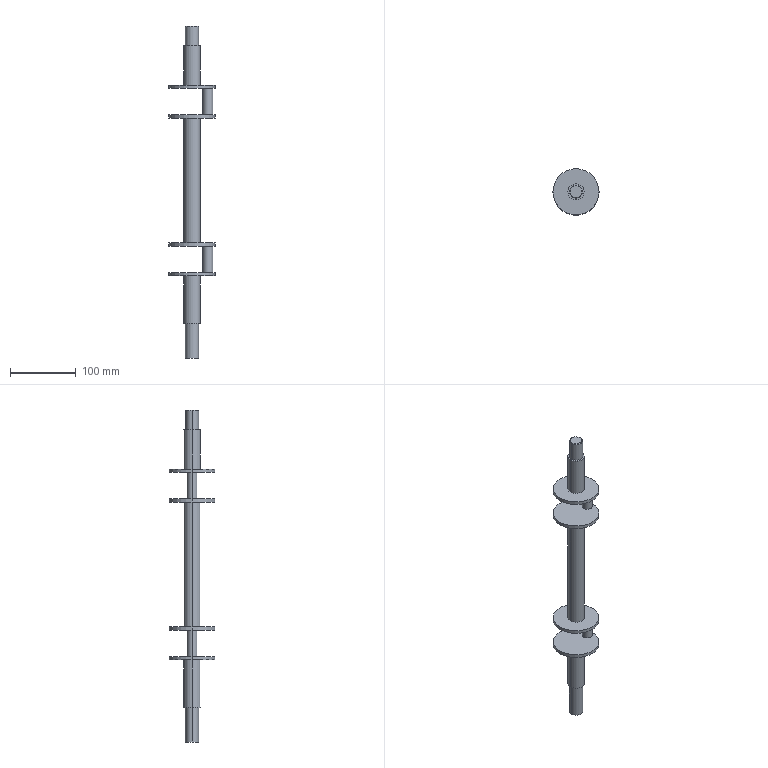Part | SolidWorks | features BaseBody 1 | 1 solid | 36 faces | box 70 x 70 x 505 mm | volume 275389 mm3 | cylinder 22 | plane 12 | cone 2 | commonest cylinder face diameters 70 x8 25 x6 15 x4 20 x4
STEP:
#1=CARTESIAN_POINT('',(10.,0.,30.));
#2=VERTEX_POINT('',#1);
#3=CARTESIAN_POINT('',(-10.,0.,30.));
#4=VERTEX_POINT('',#3);
#5=CARTESIAN_POINT('',(0.,0.,30.));
#6=DIRECTION('',(0.,0.,-1.));
#7=DIRECTION('',(1.,0.,0.));
#8=AXIS2_PLACEMENT_3D('',#5,#6,#7);
#9=CIRCLE('',#8,10.);
#10=EDGE_CURVE('',#2,#4,#9,.T.);
#11=ORIENTED_EDGE('',*,*,#10,.T.);
#12=CARTESIAN_POINT('',(-10.,0.,-22.));
#13=VERTEX_POINT('',#12);
#14=CARTESIAN_POINT('',(-10.,0.,0.));
#15=DIRECTION('',(0.,0.,-1.));
#16=VECTOR('',#15,1000.);
#17=LINE('',#14,#16);
#18=EDGE_CURVE('',#4,#13,#17,.T.);
#19=ORIENTED_EDGE('',*,*,#18,.T.);
#20=CARTESIAN_POINT('',(10.,0.,-22.));
#21=VERTEX_POINT('',#20);
#22=CARTESIAN_POINT('',(0.,0.,-22.));
#23=DIRECTION('',(0.,0.,-1.));
#24=DIRECTION('',(1.,0.,0.));
#25=AXIS2_PLACEMENT_3D('',#22,#23,#24);
#26=CIRCLE('',#25,10.);
#27=EDGE_CURVE('',#21,#13,#26,.T.);
#28=ORIENTED_EDGE('',*,*,#27,.F.);
#29=CARTESIAN_POINT('',(10.,0.,0.));
#30=DIRECTION('',(0.,0.,-1.));
#31=VECTOR('',#30,1000.);
#32=LINE('',#29,#31);
#33=EDGE_CURVE('',#2,#21,#32,.T.);
#34=ORIENTED_EDGE('',*,*,#33,.F.);
#35=EDGE_LOOP('',(#11,#19,#28,#34));
#36=FACE_OUTER_BOUND('',#35,.T.);
#37=CARTESIAN_POINT('',(0.,0.,0.));
#38=DIRECTION('',(0.,0.,-1.));
#39=DIRECTION('',(1.,0.,0.));
#40=AXIS2_PLACEMENT_3D('',#37,#38,#39);
#41=CYLINDRICAL_SURFACE('',#40,10.);
#42=ADVANCED_FACE('',(#36),#41,.T.);
#43=CARTESIAN_POINT('',(-9.,0.,483.));
#44=VERTEX_POINT('',#43);
#45=CARTESIAN_POINT('',(9.,0.,483.));
#46=VERTEX_POINT('',#45);
#47=CARTESIAN_POINT('',(0.,0.,483.));
#48=DIRECTION('',(0.,0.,-1.));
#49=DIRECTION('',(-1.,0.,0.));
#50=AXIS2_PLACEMENT_3D('',#47,#48,#49);
#51=CIRCLE('',#50,9.);
#52=EDGE_CURVE('',#44,#46,#51,.T.);
#53=ORIENTED_EDGE('',*,*,#52,.T.);
#54=CARTESIAN_POINT('',(10.,0.,482.));
#55=VERTEX_POINT('',#54);
#56=CARTESIAN_POINT('',(9.5,0.,482.5));
#57=DIRECTION('',(0.7071,0.,-0.7071));
#58=VECTOR('',#57,1000.);
#59=LINE('',#56,#58);
#60=EDGE_CURVE('',#46,#55,#59,.T.);
#61=ORIENTED_EDGE('',*,*,#60,.T.);
#62=CARTESIAN_POINT('',(-10.,0.,482.));
#63=VERTEX_POINT('',#62);
#64=CARTESIAN_POINT('',(0.,0.,482.));
#65=DIRECTION('',(0.,0.,1.));
#66=DIRECTION('',(-1.,0.,0.));
#67=AXIS2_PLACEMENT_3D('',#64,#65,#66);
#68=CIRCLE('',#67,10.);
#69=EDGE_CURVE('',#55,#63,#68,.T.);
#70=ORIENTED_EDGE('',*,*,#69,.T.);
#71=CARTESIAN_POINT('',(-9.5,0.,482.5));
#72=DIRECTION('',(-0.7071,0.,-0.7071));
#73=VECTOR('',#72,1000.);
#74=LINE('',#71,#73);
#75=EDGE_CURVE('',#44,#63,#74,.T.);
#76=ORIENTED_EDGE('',*,*,#75,.F.);
#77=EDGE_LOOP('',(#53,#61,#70,#76));
#78=FACE_OUTER_BOUND('',#77,.T.);
#79=CARTESIAN_POINT('',(0.,0.,482.5));
#80=DIRECTION('',(0.,0.,-1.));
#81=DIRECTION('',(-1.,0.,0.));
#82=AXIS2_PLACEMENT_3D('',#79,#80,#81);
#83=CONICAL_SURFACE('',#82,9.5,0.7854);
#84=ADVANCED_FACE('',(#78),#83,.T.);
#85=CARTESIAN_POINT('',(-10.,0.,453.));
#86=VERTEX_POINT('',#85);
#87=CARTESIAN_POINT('',(10.,0.,453.));
#88=VERTEX_POINT('',#87);
#89=CARTESIAN_POINT('',(0.,0.,453.));
#90=DIRECTION('',(0.,0.,1.));
#91=DIRECTION('',(-1.,0.,0.));
#92=AXIS2_PLACEMENT_3D('',#89,#90,#91);
#93=CIRCLE('',#92,10.);
#94=EDGE_CURVE('',#86,#88,#93,.T.);
#95=ORIENTED_EDGE('',*,*,#94,.T.);
#96=CARTESIAN_POINT('',(10.,0.,483.));
#97=DIRECTION('',(0.,0.,1.));
#98=VECTOR('',#97,1000.);
#99=LINE('',#96,#98);
#100=EDGE_CURVE('',#88,#55,#99,.T.);
#101=ORIENTED_EDGE('',*,*,#100,.T.);
#102=CARTESIAN_POINT('',(0.,0.,482.));
#103=DIRECTION('',(0.,0.,1.));
#104=DIRECTION('',(-1.,0.,0.));
#105=AXIS2_PLACEMENT_3D('',#102,#103,#104);
#106=CIRCLE('',#105,10.);
#107=EDGE_CURVE('',#63,#55,#106,.T.);
#108=ORIENTED_EDGE('',*,*,#107,.F.);
#109=CARTESIAN_POINT('',(-10.,0.,483.));
#110=DIRECTION('',(0.,0.,1.));
#111=VECTOR('',#110,1000.);
#112=LINE('',#109,#111);
#113=EDGE_CURVE('',#86,#63,#112,.T.);
#114=ORIENTED_EDGE('',*,*,#113,.F.);
#115=EDGE_LOOP('',(#95,#101,#108,#114));
#116=FACE_OUTER_BOUND('',#115,.T.);
#117=CARTESIAN_POINT('',(0.,0.,483.));
#118=DIRECTION('',(0.,0.,1.));
#119=DIRECTION('',(-1.,0.,0.));
#120=AXIS2_PLACEMENT_3D('',#117,#118,#119);
#121=CYLINDRICAL_SURFACE('',#120,10.);
#122=ADVANCED_FACE('',(#116),#121,.T.);
#123=CARTESIAN_POINT('',(-12.5,0.,453.));
#124=VERTEX_POINT('',#123);
#125=CARTESIAN_POINT('',(12.5,0.,453.));
#126=VERTEX_POINT('',#125);
#127=CARTESIAN_POINT('',(0.,0.,453.));
#128=DIRECTION('',(0.,0.,-1.));
#129=DIRECTION('',(-1.,0.,0.));
#130=AXIS2_PLACEMENT_3D('',#127,#128,#129);
#131=CIRCLE('',#130,12.5);
#132=EDGE_CURVE('',#124,#126,#131,.T.);
#133=ORIENTED_EDGE('',*,*,#132,.T.);
#134=CARTESIAN_POINT('',(12.5,0.,393.));
#135=VERTEX_POINT('',#134);
#136=CARTESIAN_POINT('',(12.5,0.,393.));
#137=DIRECTION('',(0.,0.,-1.));
#138=VECTOR('',#137,1000.);
#139=LINE('',#136,#138);
#140=EDGE_CURVE('',#126,#135,#139,.T.);
#141=ORIENTED_EDGE('',*,*,#140,.T.);
#142=CARTESIAN_POINT('',(-12.5,0.,393.));
#143=VERTEX_POINT('',#142);
#144=CARTESIAN_POINT('',(0.,0.,393.));
#145=DIRECTION('',(0.,0.,-1.));
#146=DIRECTION('',(-1.,0.,0.));
#147=AXIS2_PLACEMENT_3D('',#144,#145,#146);
#148=CIRCLE('',#147,12.5);
#149=EDGE_CURVE('',#143,#135,#148,.T.);
#150=ORIENTED_EDGE('',*,*,#149,.F.);
#151=CARTESIAN_POINT('',(-12.5,0.,393.));
#152=DIRECTION('',(0.,0.,-1.));
#153=VECTOR('',#152,1000.);
#154=LINE('',#151,#153);
#155=EDGE_CURVE('',#124,#143,#154,.T.);
#156=ORIENTED_EDGE('',*,*,#155,.F.);
#157=EDGE_LOOP('',(#133,#141,#150,#156));
#158=FACE_OUTER_BOUND('',#157,.T.);
#159=CARTESIAN_POINT('',(0.,0.,393.));
#160=DIRECTION('',(0.,0.,-1.));
#161=DIRECTION('',(-1.,0.,0.));
#162=AXIS2_PLACEMENT_3D('',#159,#160,#161);
#163=CYLINDRICAL_SURFACE('',#162,12.5);
#164=ADVANCED_FACE('',(#158),#163,.T.);
#165=CARTESIAN_POINT('',(35.,0.,393.));
#166=VERTEX_POINT('',#165);
#167=CARTESIAN_POINT('',(-35.,0.,393.));
#168=VERTEX_POINT('',#167);
#169=CARTESIAN_POINT('',(0.,0.,393.));
#170=DIRECTION('',(0.,0.,1.));
#171=DIRECTION('',(-1.,0.,0.));
#172=AXIS2_PLACEMENT_3D('',#169,#170,#171);
#173=CIRCLE('',#172,35.);
#174=EDGE_CURVE('',#166,#168,#173,.T.);
#175=ORIENTED_EDGE('',*,*,#174,.F.);
#176=CARTESIAN_POINT('',(35.,0.,388.));
#177=VERTEX_POINT('',#176);
#178=CARTESIAN_POINT('',(35.,0.,388.));
#179=DIRECTION('',(0.,0.,-1.));
#180=VECTOR('',#179,1000.);
#181=LINE('',#178,#180);
#182=EDGE_CURVE('',#166,#177,#181,.T.);
#183=ORIENTED_EDGE('',*,*,#182,.T.);
#184=CARTESIAN_POINT('',(-35.,0.,388.));
#185=VERTEX_POINT('',#184);
#186=CARTESIAN_POINT('',(0.,0.,388.));
#187=DIRECTION('',(0.,0.,-1.));
#188=DIRECTION('',(-1.,0.,0.));
#189=AXIS2_PLACEMENT_3D('',#186,#187,#188);
#190=CIRCLE('',#189,35.);
#191=EDGE_CURVE('',#185,#177,#190,.T.);
#192=ORIENTED_EDGE('',*,*,#191,.F.);
#193=CARTESIAN_POINT('',(-35.,0.,388.));
#194=DIRECTION('',(0.,0.,-1.));
#195=VECTOR('',#194,1000.);
#196=LINE('',#193,#195);
#197=EDGE_CURVE('',#168,#185,#196,.T.);
#198=ORIENTED_EDGE('',*,*,#197,.F.);
#199=EDGE_LOOP('',(#175,#183,#192,#198));
#200=FACE_OUTER_BOUND('',#199,.T.);
#201=CARTESIAN_POINT('',(0.,0.,388.));
#202=DIRECTION('',(0.,0.,-1.));
#203=DIRECTION('',(-1.,0.,0.));
#204=AXIS2_PLACEMENT_3D('',#201,#202,#203);
#205=CYLINDRICAL_SURFACE('',#204,35.);
#206=ADVANCED_FACE('',(#200),#205,.T.);
#207=CARTESIAN_POINT('',(31.5,0.,388.));
#208=VERTEX_POINT('',#207);
#209=CARTESIAN_POINT('',(16.5,0.,388.));
#210=VERTEX_POINT('',#209);
#211=CARTESIAN_POINT('',(24.,0.,388.));
#212=DIRECTION('',(0.,0.,1.));
#213=DIRECTION('',(-1.,0.,0.));
#214=AXIS2_PLACEMENT_3D('',#211,#212,#213);
#215=CIRCLE('',#214,7.5);
#216=EDGE_CURVE('',#208,#210,#215,.T.);
#217=ORIENTED_EDGE('',*,*,#216,.F.);
#218=CARTESIAN_POINT('',(31.5,0.,348.));
#219=VERTEX_POINT('',#218);
#220=CARTESIAN_POINT('',(31.5,0.,348.));
#221=DIRECTION('',(0.,0.,-1.));
#222=VECTOR('',#221,1000.);
#223=LINE('',#220,#222);
#224=EDGE_CURVE('',#208,#219,#223,.T.);
#225=ORIENTED_EDGE('',*,*,#224,.T.);
#226=CARTESIAN_POINT('',(16.5,0.,348.));
#227=VERTEX_POINT('',#226);
#228=CARTESIAN_POINT('',(24.,0.,348.));
#229=DIRECTION('',(0.,0.,-1.));
#230=DIRECTION('',(-1.,0.,0.));
#231=AXIS2_PLACEMENT_3D('',#228,#229,#230);
#232=CIRCLE('',#231,7.5);
#233=EDGE_CURVE('',#227,#219,#232,.T.);
#234=ORIENTED_EDGE('',*,*,#233,.F.);
#235=CARTESIAN_POINT('',(16.5,0.,348.));
#236=DIRECTION('',(0.,0.,-1.));
#237=VECTOR('',#236,1000.);
#238=LINE('',#235,#237);
#239=EDGE_CURVE('',#210,#227,#238,.T.);
#240=ORIENTED_EDGE('',*,*,#239,.F.);
#241=EDGE_LOOP('',(#217,#225,#234,#240));
#242=FACE_OUTER_BOUND('',#241,.T.);
#243=CARTESIAN_POINT('',(24.,0.,348.));
#244=DIRECTION('',(0.,0.,-1.));
#245=DIRECTION('',(-1.,0.,0.));
#246=AXIS2_PLACEMENT_3D('',#243,#244,#245);
#247=CYLINDRICAL_SURFACE('',#246,7.5);
#248=ADVANCED_FACE('',(#242),#247,.T.);
#249=CARTESIAN_POINT('',(35.,0.,348.));
#250=VERTEX_POINT('',#249);
#251=CARTESIAN_POINT('',(-35.,0.,348.));
#252=VERTEX_POINT('',#251);
#253=CARTESIAN_POINT('',(0.,0.,348.));
#254=DIRECTION('',(0.,0.,1.));
#255=DIRECTION('',(-1.,0.,0.));
#256=AXIS2_PLACEMENT_3D('',#253,#254,#255);
#257=CIRCLE('',#256,35.);
#258=EDGE_CURVE('',#250,#252,#257,.T.);
#259=ORIENTED_EDGE('',*,*,#258,.F.);
#260=CARTESIAN_POINT('',(35.,0.,343.));
#261=VERTEX_POINT('',#260);
#262=CARTESIAN_POINT('',(35.,0.,343.));
#263=DIRECTION('',(0.,0.,-1.));
#264=VECTOR('',#263,1000.);
#265=LINE('',#262,#264);
#266=EDGE_CURVE('',#250,#261,#265,.T.);
#267=ORIENTED_EDGE('',*,*,#266,.T.);
#268=CARTESIAN_POINT('',(-35.,0.,343.));
#269=VERTEX_POINT('',#268);
#270=CARTESIAN_POINT('',(0.,0.,343.));
#271=DIRECTION('',(0.,0.,-1.));
#272=DIRECTION('',(-1.,0.,0.));
#273=AXIS2_PLACEMENT_3D('',#270,#271,#272);
#274=CIRCLE('',#273,35.);
#275=EDGE_CURVE('',#269,#261,#274,.T.);
#276=ORIENTED_EDGE('',*,*,#275,.F.);
#277=CARTESIAN_POINT('',(-35.,0.,343.));
#278=DIRECTION('',(0.,0.,-1.));
#279=VECTOR('',#278,1000.);
#280=LINE('',#277,#279);
#281=EDGE_CURVE('',#252,#269,#280,.T.);
#282=ORIENTED_EDGE('',*,*,#281,.F.);
#283=EDGE_LOOP('',(#259,#267,#276,#282));
#284=FACE_OUTER_BOUND('',#283,.T.);
#285=CARTESIAN_POINT('',(0.,0.,343.));
#286=DIRECTION('',(0.,0.,-1.));
#287=DIRECTION('',(-1.,0.,0.));
#288=AXIS2_PLACEMENT_3D('',#285,#286,#287);
#289=CYLINDRICAL_SURFACE('',#288,35.);
#290=ADVANCED_FACE('',(#284),#289,.T.);
#291=CARTESIAN_POINT('',(12.5,0.,343.));
#292=VERTEX_POINT('',#291);
#293=CARTESIAN_POINT('',(-12.5,0.,343.));
#294=VERTEX_POINT('',#293);
#295=CARTESIAN_POINT('',(0.,0.,343.));
#296=DIRECTION('',(0.,0.,1.));
#297=DIRECTION('',(-1.,0.,0.));
#298=AXIS2_PLACEMENT_3D('',#295,#296,#297);
#299=CIRCLE('',#298,12.5);
#300=EDGE_CURVE('',#292,#294,#299,.T.);
#301=ORIENTED_EDGE('',*,*,#300,.F.);
#302=CARTESIAN_POINT('',(12.5,0.,153.));
#303=VERTEX_POINT('',#302);
#304=CARTESIAN_POINT('',(12.5,0.,153.));
#305=DIRECTION('',(0.,0.,-1.));
#306=VECTOR('',#305,1000.);
#307=LINE('',#304,#306);
#308=EDGE_CURVE('',#292,#303,#307,.T.);
#309=ORIENTED_EDGE('',*,*,#308,.T.);
#310=CARTESIAN_POINT('',(-12.5,0.,153.));
#311=VERTEX_POINT('',#310);
#312=CARTESIAN_POINT('',(0.,0.,153.));
#313=DIRECTION('',(0.,0.,-1.));
#314=DIRECTION('',(-1.,0.,0.));
#315=AXIS2_PLACEMENT_3D('',#312,#313,#314);
#316=CIRCLE('',#315,12.5);
#317=EDGE_CURVE('',#311,#303,#316,.T.);
#318=ORIENTED_EDGE('',*,*,#317,.F.);
#319=CARTESIAN_POINT('',(-12.5,0.,153.));
#320=DIRECTION('',(0.,0.,-1.));
#321=VECTOR('',#320,1000.);
#322=LINE('',#319,#321);
#323=EDGE_CURVE('',#294,#311,#322,.T.);
#324=ORIENTED_EDGE('',*,*,#323,.F.);
#325=EDGE_LOOP('',(#301,#309,#318,#324));
#326=FACE_OUTER_BOUND('',#325,.T.);
#327=CARTESIAN_POINT('',(0.,0.,153.));
#328=DIRECTION('',(0.,0.,-1.));
#329=DIRECTION('',(-1.,0.,0.));
#330=AXIS2_PLACEMENT_3D('',#327,#328,#329);
#331=CYLINDRICAL_SURFACE('',#330,12.5);
#332=ADVANCED_FACE('',(#326),#331,.T.);
#333=CARTESIAN_POINT('',(35.,0.,153.));
#334=VERTEX_POINT('',#333);
#335=CARTESIAN_POINT('',(-35.,0.,153.));
#336=VERTEX_POINT('',#335);
#337=CARTESIAN_POINT('',(0.,0.,153.));
#338=DIRECTION('',(0.,0.,1.));
#339=DIRECTION('',(-1.,0.,0.));
#340=AXIS2_PLACEMENT_3D('',#337,#338,#339);
#341=CIRCLE('',#340,35.);
#342=EDGE_CURVE('',#334,#336,#341,.T.);
#343=ORIENTED_EDGE('',*,*,#342,.F.);
#344=CARTESIAN_POINT('',(35.,0.,148.));
#345=VERTEX_POINT('',#344);
#346=CARTESIAN_POINT('',(35.,0.,148.));
#347=DIRECTION('',(0.,0.,-1.));
#348=VECTOR('',#347,1000.);
#349=LINE('',#346,#348);
#350=EDGE_CURVE('',#334,#345,#349,.T.);
#351=ORIENTED_EDGE('',*,*,#350,.T.);
#352=CARTESIAN_POINT('',(-35.,0.,148.));
#353=VERTEX_POINT('',#352);
#354=CARTESIAN_POINT('',(0.,0.,148.));
#355=DIRECTION('',(0.,0.,-1.));
#356=DIRECTION('',(-1.,0.,0.));
#357=AXIS2_PLACEMENT_3D('',#354,#355,#356);
#358=CIRCLE('',#357,35.);
#359=EDGE_CURVE('',#353,#345,#358,.T.);
#360=ORIENTED_EDGE('',*,*,#359,.F.);
#361=CARTESIAN_POINT('',(-35.,0.,148.));
#362=DIRECTION('',(0.,0.,-1.));
#363=VECTOR('',#362,1000.);
#364=LINE('',#361,#363);
#365=EDGE_CURVE('',#336,#353,#364,.T.);
#366=ORIENTED_EDGE('',*,*,#365,.F.);
#367=EDGE_LOOP('',(#343,#351,#360,#366));
#368=FACE_OUTER_BOUND('',#367,.T.);
#369=CARTESIAN_POINT('',(0.,0.,148.));
#370=DIRECTION('',(0.,0.,-1.));
#371=DIRECTION('',(-1.,0.,0.));
#372=AXIS2_PLACEMENT_3D('',#369,#370,#371);
#373=CYLINDRICAL_SURFACE('',#372,35.);
#374=ADVANCED_FACE('',(#368),#373,.T.);
#375=CARTESIAN_POINT('',(31.5,0.,148.));
#376=VERTEX_POINT('',#375);
#377=CARTESIAN_POINT('',(16.5,0.,148.));
#378=VERTEX_POINT('',#377);
#379=CARTESIAN_POINT('',(24.,0.,148.));
#380=DIRECTION('',(0.,0.,1.));
#381=DIRECTION('',(-1.,0.,0.));
#382=AXIS2_PLACEMENT_3D('',#379,#380,#381);
#383=CIRCLE('',#382,7.5);
#384=EDGE_CURVE('',#376,#378,#383,.T.);
#385=ORIENTED_EDGE('',*,*,#384,.F.);
#386=CARTESIAN_POINT('',(31.5,0.,108.));
#387=VERTEX_POINT('',#386);
#388=CARTESIAN_POINT('',(31.5,0.,108.));
#389=DIRECTION('',(0.,0.,-1.));
#390=VECTOR('',#389,1000.);
#391=LINE('',#388,#390);
#392=EDGE_CURVE('',#376,#387,#391,.T.);
#393=ORIENTED_EDGE('',*,*,#392,.T.);
#394=CARTESIAN_POINT('',(16.5,0.,108.));
#395=VERTEX_POINT('',#394);
#396=CARTESIAN_POINT('',(24.,0.,108.));
#397=DIRECTION('',(0.,0.,-1.));
#398=DIRECTION('',(-1.,0.,0.));
#399=AXIS2_PLACEMENT_3D('',#396,#397,#398);
#400=CIRCLE('',#399,7.5);
#401=EDGE_CURVE('',#395,#387,#400,.T.);
#402=ORIENTED_EDGE('',*,*,#401,.F.);
#403=CARTESIAN_POINT('',(16.5,0.,108.));
#404=DIRECTION('',(0.,0.,-1.));
#405=VECTOR('',#404,1000.);
#406=LINE('',#403,#405);
#407=EDGE_CURVE('',#378,#395,#406,.T.);
#408=ORIENTED_EDGE('',*,*,#407,.F.);
#409=EDGE_LOOP('',(#385,#393,#402,#408));
#410=FACE_OUTER_BOUND('',#409,.T.);
#411=CARTESIAN_POINT('',(24.,0.,108.));
#412=DIRECTION('',(0.,0.,-1.));
#413=DIRECTION('',(-1.,0.,0.));
#414=AXIS2_PLACEMENT_3D('',#411,#412,#413);
#415=CYLINDRICAL_SURFACE('',#414,7.5);
#416=ADVANCED_FACE('',(#410),#415,.T.);
#417=CARTESIAN_POINT('',(35.,0.,108.));
#418=VERTEX_POINT('',#417);
#419=CARTESIAN_POINT('',(-35.,0.,108.));
#420=VERTEX_POINT('',#419);
#421=CARTESIAN_POINT('',(0.,0.,108.));
#422=DIRECTION('',(0.,0.,1.));
#423=DIRECTION('',(-1.,0.,0.));
#424=AXIS2_PLACEMENT_3D('',#421,#422,#423);
#425=CIRCLE('',#424,35.);
#426=EDGE_CURVE('',#418,#420,#425,.T.);
#427=ORIENTED_EDGE('',*,*,#426,.F.);
#428=CARTESIAN_POINT('',(35.,0.,103.));
#429=VERTEX_POINT('',#428);
#430=CARTESIAN_POINT('',(35.,0.,103.));
#431=DIRECTION('',(0.,0.,-1.));
#432=VECTOR('',#431,1000.);
#433=LINE('',#430,#432);
#434=EDGE_CURVE('',#418,#429,#433,.T.);
#435=ORIENTED_EDGE('',*,*,#434,.T.);
#436=CARTESIAN_POINT('',(-35.,0.,103.));
#437=VERTEX_POINT('',#436);
#438=CARTESIAN_POINT('',(0.,0.,103.));
#439=DIRECTION('',(0.,0.,-1.));
#440=DIRECTION('',(-1.,0.,0.));
#441=AXIS2_PLACEMENT_3D('',#438,#439,#440);
#442=CIRCLE('',#441,35.);
#443=EDGE_CURVE('',#437,#429,#442,.T.);
#444=ORIENTED_EDGE('',*,*,#443,.F.);
#445=CARTESIAN_POINT('',(-35.,0.,103.));
#446=DIRECTION('',(0.,0.,-1.));
#447=VECTOR('',#446,1000.);
#448=LINE('',#445,#447);
#449=EDGE_CURVE('',#420,#437,#448,.T.);
#450=ORIENTED_EDGE('',*,*,#449,.F.);
#451=EDGE_LOOP('',(#427,#435,#444,#450));
#452=FACE_OUTER_BOUND('',#451,.T.);
#453=CARTESIAN_POINT('',(0.,0.,103.));
#454=DIRECTION('',(0.,0.,-1.));
#455=DIRECTION('',(-1.,0.,0.));
#456=AXIS2_PLACEMENT_3D('',#453,#454,#455);
#457=CYLINDRICAL_SURFACE('',#456,35.);
#458=ADVANCED_FACE('',(#452),#457,.T.);
#459=CARTESIAN_POINT('',(12.5,0.,103.));
#460=VERTEX_POINT('',#459);
#461=CARTESIAN_POINT('',(-12.5,0.,103.));
#462=VERTEX_POINT('',#461);
#463=CARTESIAN_POINT('',(0.,0.,103.));
#464=DIRECTION('',(0.,0.,1.));
#465=DIRECTION('',(-1.,0.,0.));
#466=AXIS2_PLACEMENT_3D('',#463,#464,#465);
#467=CIRCLE('',#466,12.5);
#468=EDGE_CURVE('',#460,#462,#467,.T.);
#469=ORIENTED_EDGE('',*,*,#468,.F.);
#470=CARTESIAN_POINT('',(12.5,0.,30.));
#471=VERTEX_POINT('',#470);
#472=CARTESIAN_POINT('',(12.5,0.,0.));
#473=DIRECTION('',(0.,0.,-1.));
#474=VECTOR('',#473,1000.);
#475=LINE('',#472,#474);
#476=EDGE_CURVE('',#460,#471,#475,.T.);
#477=ORIENTED_EDGE('',*,*,#476,.T.);
#478=CARTESIAN_POINT('',(-12.5,0.,30.));
#479=VERTEX_POINT('',#478);
#480=CARTESIAN_POINT('',(0.,0.,30.));
#481=DIRECTION('',(0.,0.,1.));
#482=DIRECTION('',(-1.,0.,0.));
#483=AXIS2_PLACEMENT_3D('',#480,#481,#482);
#484=CIRCLE('',#483,12.5);
#485=EDGE_CURVE('',#471,#479,#484,.T.);
#486=ORIENTED_EDGE('',*,*,#485,.T.);
#487=CARTESIAN_POINT('',(-12.5,0.,0.));
#488=DIRECTION('',(0.,0.,-1.));
#489=VECTOR('',#488,1000.);
#490=LINE('',#487,#489);
#491=EDGE_CURVE('',#462,#479,#490,.T.);
#492=ORIENTED_EDGE('',*,*,#491,.F.);
#493=EDGE_LOOP('',(#469,#477,#486,#492));
#494=FACE_OUTER_BOUND('',#493,.T.);
#495=CARTESIAN_POINT('',(0.,0.,0.));
#496=DIRECTION('',(0.,0.,-1.));
#497=DIRECTION('',(-1.,0.,0.));
#498=AXIS2_PLACEMENT_3D('',#495,#496,#497);
#499=CYLINDRICAL_SURFACE('',#498,12.5);
#500=ADVANCED_FACE('',(#494),#499,.T.);
#501=ORIENTED_EDGE('',*,*,#27,.T.);
#502=CARTESIAN_POINT('',(0.,0.,-22.));
#503=DIRECTION('',(0.,0.,-1.));
#504=DIRECTION('',(1.,0.,0.));
#505=AXIS2_PLACEMENT_3D('',#502,#503,#504);
#506=CIRCLE('',#505,10.);
#507=EDGE_CURVE('',#13,#21,#506,.T.);
#508=ORIENTED_EDGE('',*,*,#507,.T.);
#509=EDGE_LOOP('',(#501,#508));
#510=FACE_OUTER_BOUND('',#509,.T.);
#511=CARTESIAN_POINT('',(0.,0.,-22.));
#512=DIRECTION('',(0.,0.,1.));
#513=DIRECTION('',(1.,0.,0.));
#514=AXIS2_PLACEMENT_3D('',#511,#512,#513);
#515=PLANE('',#514);
#516=ADVANCED_FACE('',(#510),#515,.F.);
#517=ORIENTED_EDGE('',*,*,#10,.F.);
#518=CARTESIAN_POINT('',(0.,0.,30.));
#519=DIRECTION('',(0.,0.,-1.));
#520=DIRECTION('',(1.,0.,0.));
#521=AXIS2_PLACEMENT_3D('',#518,#519,#520);
#522=CIRCLE('',#521,10.);
#523=EDGE_CURVE('',#4,#2,#522,.T.);
#524=ORIENTED_EDGE('',*,*,#523,.F.);
#525=EDGE_LOOP('',(#517,#524));
#526=FACE_BOUND('',#525,.T.);
#527=CARTESIAN_POINT('',(0.,0.,30.));
#528=DIRECTION('',(0.,0.,1.));
#529=DIRECTION('',(-1.,0.,0.));
#530=AXIS2_PLACEMENT_3D('',#527,#528,#529);
#531=CIRCLE('',#530,12.5);
#532=EDGE_CURVE('',#479,#471,#531,.T.);
#533=ORIENTED_EDGE('',*,*,#532,.F.);
#534=ORIENTED_EDGE('',*,*,#485,.F.);
#535=EDGE_LOOP('',(#533,#534));
#536=FACE_OUTER_BOUND('',#535,.T.);
#537=CARTESIAN_POINT('',(0.,0.,30.));
#538=DIRECTION('',(0.,0.,1.));
#539=DIRECTION('',(1.,0.,0.));
#540=AXIS2_PLACEMENT_3D('',#537,#538,#539);
#541=PLANE('',#540);
#542=ADVANCED_FACE('',(#526,#536),#541,.F.);
#543=ORIENTED_EDGE('',*,*,#52,.F.);
#544=CARTESIAN_POINT('',(0.,0.,483.));
#545=DIRECTION('',(0.,0.,-1.));
#546=DIRECTION('',(-1.,0.,0.));
#547=AXIS2_PLACEMENT_3D('',#544,#545,#546);
#548=CIRCLE('',#547,9.);
#549=EDGE_CURVE('',#46,#44,#548,.T.);
#550=ORIENTED_EDGE('',*,*,#549,.F.);
#551=EDGE_LOOP('',(#543,#550));
#552=FACE_OUTER_BOUND('',#551,.T.);
#553=CARTESIAN_POINT('',(0.,0.,483.));
#554=DIRECTION('',(0.,0.,1.));
#555=DIRECTION('',(1.,0.,0.));
#556=AXIS2_PLACEMENT_3D('',#553,#554,#555);
#557=PLANE('',#556);
#558=ADVANCED_FACE('',(#552),#557,.T.);
#559=ORIENTED_EDGE('',*,*,#94,.F.);
#560=CARTESIAN_POINT('',(0.,0.,453.));
#561=DIRECTION('',(0.,0.,1.));
#562=DIRECTION('',(-1.,0.,0.));
#563=AXIS2_PLACEMENT_3D('',#560,#561,#562);
#564=CIRCLE('',#563,10.);
#565=EDGE_CURVE('',#88,#86,#564,.T.);
#566=ORIENTED_EDGE('',*,*,#565,.F.);
#567=EDGE_LOOP('',(#559,#566));
#568=FACE_BOUND('',#567,.T.);
#569=ORIENTED_EDGE('',*,*,#132,.F.);
#570=CARTESIAN_POINT('',(0.,0.,453.));
#571=DIRECTION('',(0.,0.,-1.));
#572=DIRECTION('',(-1.,0.,0.));
#573=AXIS2_PLACEMENT_3D('',#570,#571,#572);
#574=CIRCLE('',#573,12.5);
#575=EDGE_CURVE('',#126,#124,#574,.T.);
#576=ORIENTED_EDGE('',*,*,#575,.F.);
#577=EDGE_LOOP('',(#569,#576));
#578=FACE_OUTER_BOUND('',#577,.T.);
#579=CARTESIAN_POINT('',(0.,0.,453.));
#580=DIRECTION('',(0.,0.,1.));
#581=DIRECTION('',(1.,0.,0.));
#582=AXIS2_PLACEMENT_3D('',#579,#580,#581);
#583=PLANE('',#582);
#584=ADVANCED_FACE('',(#568,#578),#583,.T.);
#585=CARTESIAN_POINT('',(24.,0.,388.));
#586=DIRECTION('',(0.,0.,1.));
#587=DIRECTION('',(-1.,0.,0.));
#588=AXIS2_PLACEMENT_3D('',#585,#586,#587);
#589=CIRCLE('',#588,7.5);
#590=EDGE_CURVE('',#210,#208,#589,.T.);
#591=ORIENTED_EDGE('',*,*,#590,.T.);
#592=ORIENTED_EDGE('',*,*,#216,.T.);
#593=EDGE_LOOP('',(#591,#592));
#594=FACE_BOUND('',#593,.T.);
#595=ORIENTED_EDGE('',*,*,#191,.T.);
#596=CARTESIAN_POINT('',(0.,0.,388.));
#597=DIRECTION('',(0.,0.,-1.));
#598=DIRECTION('',(-1.,0.,0.));
#599=AXIS2_PLACEMENT_3D('',#596,#597,#598);
#600=CIRCLE('',#599,35.);
#601=EDGE_CURVE('',#177,#185,#600,.T.);
#602=ORIENTED_EDGE('',*,*,#601,.T.);
#603=EDGE_LOOP('',(#595,#602));
#604=FACE_OUTER_BOUND('',#603,.T.);
#605=CARTESIAN_POINT('',(0.,0.,388.));
#606=DIRECTION('',(0.,0.,1.));
#607=DIRECTION('',(1.,0.,0.));
#608=AXIS2_PLACEMENT_3D('',#605,#606,#607);
#609=PLANE('',#608);
#610=ADVANCED_FACE('',(#594,#604),#609,.F.);
#611=ORIENTED_EDGE('',*,*,#149,.T.);
#612=CARTESIAN_POINT('',(0.,0.,393.));
#613=DIRECTION('',(0.,0.,-1.));
#614=DIRECTION('',(-1.,0.,0.));
#615=AXIS2_PLACEMENT_3D('',#612,#613,#614);
#616=CIRCLE('',#615,12.5);
#617=EDGE_CURVE('',#135,#143,#616,.T.);
#618=ORIENTED_EDGE('',*,*,#617,.T.);
#619=EDGE_LOOP('',(#611,#618));
#620=FACE_BOUND('',#619,.T.);
#621=CARTESIAN_POINT('',(0.,0.,393.));
#622=DIRECTION('',(0.,0.,1.));
#623=DIRECTION('',(-1.,0.,0.));
#624=AXIS2_PLACEMENT_3D('',#621,#622,#623);
#625=CIRCLE('',#624,35.);
#626=EDGE_CURVE('',#168,#166,#625,.T.);
#627=ORIENTED_EDGE('',*,*,#626,.T.);
#628=ORIENTED_EDGE('',*,*,#174,.T.);
#629=EDGE_LOOP('',(#627,#628));
#630=FACE_OUTER_BOUND('',#629,.T.);
#631=CARTESIAN_POINT('',(0.,0.,393.));
#632=DIRECTION('',(0.,0.,1.));
#633=DIRECTION('',(1.,0.,0.));
#634=AXIS2_PLACEMENT_3D('',#631,#632,#633);
#635=PLANE('',#634);
#636=ADVANCED_FACE('',(#620,#630),#635,.T.);
#637=CARTESIAN_POINT('',(0.,0.,343.));
#638=DIRECTION('',(0.,0.,1.));
#639=DIRECTION('',(-1.,0.,0.));
#640=AXIS2_PLACEMENT_3D('',#637,#638,#639);
#641=CIRCLE('',#640,12.5);
#642=EDGE_CURVE('',#294,#292,#641,.T.);
#643=ORIENTED_EDGE('',*,*,#642,.T.);
#644=ORIENTED_EDGE('',*,*,#300,.T.);
#645=EDGE_LOOP('',(#643,#644));
#646=FACE_BOUND('',#645,.T.);
#647=ORIENTED_EDGE('',*,*,#275,.T.);
#648=CARTESIAN_POINT('',(0.,0.,343.));
#649=DIRECTION('',(0.,0.,-1.));
#650=DIRECTION('',(-1.,0.,0.));
#651=AXIS2_PLACEMENT_3D('',#648,#649,#650);
#652=CIRCLE('',#651,35.);
#653=EDGE_CURVE('',#261,#269,#652,.T.);
#654=ORIENTED_EDGE('',*,*,#653,.T.);
#655=EDGE_LOOP('',(#647,#654));
#656=FACE_OUTER_BOUND('',#655,.T.);
#657=CARTESIAN_POINT('',(0.,0.,343.));
#658=DIRECTION('',(0.,0.,1.));
#659=DIRECTION('',(1.,0.,0.));
#660=AXIS2_PLACEMENT_3D('',#657,#658,#659);
#661=PLANE('',#660);
#662=ADVANCED_FACE('',(#646,#656),#661,.F.);
#663=ORIENTED_EDGE('',*,*,#233,.T.);
#664=CARTESIAN_POINT('',(24.,0.,348.));
#665=DIRECTION('',(0.,0.,-1.));
#666=DIRECTION('',(-1.,0.,0.));
#667=AXIS2_PLACEMENT_3D('',#664,#665,#666);
#668=CIRCLE('',#667,7.5);
#669=EDGE_CURVE('',#219,#227,#668,.T.);
#670=ORIENTED_EDGE('',*,*,#669,.T.);
#671=EDGE_LOOP('',(#663,#670));
#672=FACE_BOUND('',#671,.T.);
#673=CARTESIAN_POINT('',(0.,0.,348.));
#674=DIRECTION('',(0.,0.,1.));
#675=DIRECTION('',(-1.,0.,0.));
#676=AXIS2_PLACEMENT_3D('',#673,#674,#675);
#677=CIRCLE('',#676,35.);
#678=EDGE_CURVE('',#252,#250,#677,.T.);
#679=ORIENTED_EDGE('',*,*,#678,.T.);
#680=ORIENTED_EDGE('',*,*,#258,.T.);
#681=EDGE_LOOP('',(#679,#680));
#682=FACE_OUTER_BOUND('',#681,.T.);
#683=CARTESIAN_POINT('',(0.,0.,348.));
#684=DIRECTION('',(0.,0.,1.));
#685=DIRECTION('',(1.,0.,0.));
#686=AXIS2_PLACEMENT_3D('',#683,#684,#685);
#687=PLANE('',#686);
#688=ADVANCED_FACE('',(#672,#682),#687,.T.);
#689=CARTESIAN_POINT('',(24.,0.,148.));
#690=DIRECTION('',(0.,0.,1.));
#691=DIRECTION('',(-1.,0.,0.));
#692=AXIS2_PLACEMENT_3D('',#689,#690,#691);
#693=CIRCLE('',#692,7.5);
#694=EDGE_CURVE('',#378,#376,#693,.T.);
#695=ORIENTED_EDGE('',*,*,#694,.T.);
#696=ORIENTED_EDGE('',*,*,#384,.T.);
#697=EDGE_LOOP('',(#695,#696));
#698=FACE_BOUND('',#697,.T.);
#699=ORIENTED_EDGE('',*,*,#359,.T.);
#700=CARTESIAN_POINT('',(0.,0.,148.));
#701=DIRECTION('',(0.,0.,-1.));
#702=DIRECTION('',(-1.,0.,0.));
#703=AXIS2_PLACEMENT_3D('',#700,#701,#702);
#704=CIRCLE('',#703,35.);
#705=EDGE_CURVE('',#345,#353,#704,.T.);
#706=ORIENTED_EDGE('',*,*,#705,.T.);
#707=EDGE_LOOP('',(#699,#706));
#708=FACE_OUTER_BOUND('',#707,.T.);
#709=CARTESIAN_POINT('',(0.,0.,148.));
#710=DIRECTION('',(0.,0.,1.));
#711=DIRECTION('',(1.,0.,0.));
#712=AXIS2_PLACEMENT_3D('',#709,#710,#711);
#713=PLANE('',#712);
#714=ADVANCED_FACE('',(#698,#708),#713,.F.);
#715=ORIENTED_EDGE('',*,*,#317,.T.);
#716=CARTESIAN_POINT('',(0.,0.,153.));
#717=DIRECTION('',(0.,0.,-1.));
#718=DIRECTION('',(-1.,0.,0.));
#719=AXIS2_PLACEMENT_3D('',#716,#717,#718);
#720=CIRCLE('',#719,12.5);
#721=EDGE_CURVE('',#303,#311,#720,.T.);
#722=ORIENTED_EDGE('',*,*,#721,.T.);
#723=EDGE_LOOP('',(#715,#722));
#724=FACE_BOUND('',#723,.T.);
#725=CARTESIAN_POINT('',(0.,0.,153.));
#726=DIRECTION('',(0.,0.,1.));
#727=DIRECTION('',(-1.,0.,0.));
#728=AXIS2_PLACEMENT_3D('',#725,#726,#727);
#729=CIRCLE('',#728,35.);
#730=EDGE_CURVE('',#336,#334,#729,.T.);
#731=ORIENTED_EDGE('',*,*,#730,.T.);
#732=ORIENTED_EDGE('',*,*,#342,.T.);
#733=EDGE_LOOP('',(#731,#732));
#734=FACE_OUTER_BOUND('',#733,.T.);
#735=CARTESIAN_POINT('',(0.,0.,153.));
#736=DIRECTION('',(0.,0.,1.));
#737=DIRECTION('',(1.,0.,0.));
#738=AXIS2_PLACEMENT_3D('',#735,#736,#737);
#739=PLANE('',#738);
#740=ADVANCED_FACE('',(#724,#734),#739,.T.);
#741=CARTESIAN_POINT('',(0.,0.,103.));
#742=DIRECTION('',(0.,0.,1.));
#743=DIRECTION('',(-1.,0.,0.));
#744=AXIS2_PLACEMENT_3D('',#741,#742,#743);
#745=CIRCLE('',#744,12.5);
#746=EDGE_CURVE('',#462,#460,#745,.T.);
#747=ORIENTED_EDGE('',*,*,#746,.T.);
#748=ORIENTED_EDGE('',*,*,#468,.T.);
#749=EDGE_LOOP('',(#747,#748));
#750=FACE_BOUND('',#749,.T.);
#751=ORIENTED_EDGE('',*,*,#443,.T.);
#752=CARTESIAN_POINT('',(0.,0.,103.));
#753=DIRECTION('',(0.,0.,-1.));
#754=DIRECTION('',(-1.,0.,0.));
#755=AXIS2_PLACEMENT_3D('',#752,#753,#754);
#756=CIRCLE('',#755,35.);
#757=EDGE_CURVE('',#429,#437,#756,.T.);
#758=ORIENTED_EDGE('',*,*,#757,.T.);
#759=EDGE_LOOP('',(#751,#758));
#760=FACE_OUTER_BOUND('',#759,.T.);
#761=CARTESIAN_POINT('',(0.,0.,103.));
#762=DIRECTION('',(0.,0.,1.));
#763=DIRECTION('',(1.,0.,0.));
#764=AXIS2_PLACEMENT_3D('',#761,#762,#763);
#765=PLANE('',#764);
#766=ADVANCED_FACE('',(#750,#760),#765,.F.);
#767=ORIENTED_EDGE('',*,*,#401,.T.);
#768=CARTESIAN_POINT('',(24.,0.,108.));
#769=DIRECTION('',(0.,0.,-1.));
#770=DIRECTION('',(-1.,0.,0.));
#771=AXIS2_PLACEMENT_3D('',#768,#769,#770);
#772=CIRCLE('',#771,7.5);
#773=EDGE_CURVE('',#387,#395,#772,.T.);
#774=ORIENTED_EDGE('',*,*,#773,.T.);
#775=EDGE_LOOP('',(#767,#774));
#776=FACE_BOUND('',#775,.T.);
#777=CARTESIAN_POINT('',(0.,0.,108.));
#778=DIRECTION('',(0.,0.,1.));
#779=DIRECTION('',(-1.,0.,0.));
#780=AXIS2_PLACEMENT_3D('',#777,#778,#779);
#781=CIRCLE('',#780,35.);
#782=EDGE_CURVE('',#420,#418,#781,.T.);
#783=ORIENTED_EDGE('',*,*,#782,.T.);
#784=ORIENTED_EDGE('',*,*,#426,.T.);
#785=EDGE_LOOP('',(#783,#784));
#786=FACE_OUTER_BOUND('',#785,.T.);
#787=CARTESIAN_POINT('',(0.,0.,108.));
#788=DIRECTION('',(0.,0.,1.));
#789=DIRECTION('',(1.,0.,0.));
#790=AXIS2_PLACEMENT_3D('',#787,#788,#789);
#791=PLANE('',#790);
#792=ADVANCED_FACE('',(#776,#786),#791,.T.);
#793=ORIENTED_EDGE('',*,*,#476,.F.);
#794=ORIENTED_EDGE('',*,*,#746,.F.);
#795=ORIENTED_EDGE('',*,*,#491,.T.);
#796=ORIENTED_EDGE('',*,*,#532,.T.);
#797=EDGE_LOOP('',(#793,#794,#795,#796));
#798=FACE_OUTER_BOUND('',#797,.T.);
#799=CARTESIAN_POINT('',(0.,0.,0.));
#800=DIRECTION('',(0.,0.,-1.));
#801=DIRECTION('',(-1.,0.,0.));
#802=AXIS2_PLACEMENT_3D('',#799,#800,#801);
#803=CYLINDRICAL_SURFACE('',#802,12.5);
#804=ADVANCED_FACE('',(#798),#803,.T.);
#805=ORIENTED_EDGE('',*,*,#434,.F.);
#806=ORIENTED_EDGE('',*,*,#782,.F.);
#807=ORIENTED_EDGE('',*,*,#449,.T.);
#808=ORIENTED_EDGE('',*,*,#757,.F.);
#809=EDGE_LOOP('',(#805,#806,#807,#808));
#810=FACE_OUTER_BOUND('',#809,.T.);
#811=CARTESIAN_POINT('',(0.,0.,103.));
#812=DIRECTION('',(0.,0.,-1.));
#813=DIRECTION('',(-1.,0.,0.));
#814=AXIS2_PLACEMENT_3D('',#811,#812,#813);
#815=CYLINDRICAL_SURFACE('',#814,35.);
#816=ADVANCED_FACE('',(#810),#815,.T.);
#817=ORIENTED_EDGE('',*,*,#392,.F.);
#818=ORIENTED_EDGE('',*,*,#694,.F.);
#819=ORIENTED_EDGE('',*,*,#407,.T.);
#820=ORIENTED_EDGE('',*,*,#773,.F.);
#821=EDGE_LOOP('',(#817,#818,#819,#820));
#822=FACE_OUTER_BOUND('',#821,.T.);
#823=CARTESIAN_POINT('',(24.,0.,108.));
#824=DIRECTION('',(0.,0.,-1.));
#825=DIRECTION('',(-1.,0.,0.));
#826=AXIS2_PLACEMENT_3D('',#823,#824,#825);
#827=CYLINDRICAL_SURFACE('',#826,7.5);
#828=ADVANCED_FACE('',(#822),#827,.T.);
#829=ORIENTED_EDGE('',*,*,#350,.F.);
#830=ORIENTED_EDGE('',*,*,#730,.F.);
#831=ORIENTED_EDGE('',*,*,#365,.T.);
#832=ORIENTED_EDGE('',*,*,#705,.F.);
#833=EDGE_LOOP('',(#829,#830,#831,#832));
#834=FACE_OUTER_BOUND('',#833,.T.);
#835=CARTESIAN_POINT('',(0.,0.,148.));
#836=DIRECTION('',(0.,0.,-1.));
#837=DIRECTION('',(-1.,0.,0.));
#838=AXIS2_PLACEMENT_3D('',#835,#836,#837);
#839=CYLINDRICAL_SURFACE('',#838,35.);
#840=ADVANCED_FACE('',(#834),#839,.T.);
#841=ORIENTED_EDGE('',*,*,#308,.F.);
#842=ORIENTED_EDGE('',*,*,#642,.F.);
#843=ORIENTED_EDGE('',*,*,#323,.T.);
#844=ORIENTED_EDGE('',*,*,#721,.F.);
#845=EDGE_LOOP('',(#841,#842,#843,#844));
#846=FACE_OUTER_BOUND('',#845,.T.);
#847=CARTESIAN_POINT('',(0.,0.,153.));
#848=DIRECTION('',(0.,0.,-1.));
#849=DIRECTION('',(-1.,0.,0.));
#850=AXIS2_PLACEMENT_3D('',#847,#848,#849);
#851=CYLINDRICAL_SURFACE('',#850,12.5);
#852=ADVANCED_FACE('',(#846),#851,.T.);
#853=ORIENTED_EDGE('',*,*,#266,.F.);
#854=ORIENTED_EDGE('',*,*,#678,.F.);
#855=ORIENTED_EDGE('',*,*,#281,.T.);
#856=ORIENTED_EDGE('',*,*,#653,.F.);
#857=EDGE_LOOP('',(#853,#854,#855,#856));
#858=FACE_OUTER_BOUND('',#857,.T.);
#859=CARTESIAN_POINT('',(0.,0.,343.));
#860=DIRECTION('',(0.,0.,-1.));
#861=DIRECTION('',(-1.,0.,0.));
#862=AXIS2_PLACEMENT_3D('',#859,#860,#861);
#863=CYLINDRICAL_SURFACE('',#862,35.);
#864=ADVANCED_FACE('',(#858),#863,.T.);
#865=ORIENTED_EDGE('',*,*,#224,.F.);
#866=ORIENTED_EDGE('',*,*,#590,.F.);
#867=ORIENTED_EDGE('',*,*,#239,.T.);
#868=ORIENTED_EDGE('',*,*,#669,.F.);
#869=EDGE_LOOP('',(#865,#866,#867,#868));
#870=FACE_OUTER_BOUND('',#869,.T.);
#871=CARTESIAN_POINT('',(24.,0.,348.));
#872=DIRECTION('',(0.,0.,-1.));
#873=DIRECTION('',(-1.,0.,0.));
#874=AXIS2_PLACEMENT_3D('',#871,#872,#873);
#875=CYLINDRICAL_SURFACE('',#874,7.5);
#876=ADVANCED_FACE('',(#870),#875,.T.);
#877=ORIENTED_EDGE('',*,*,#182,.F.);
#878=ORIENTED_EDGE('',*,*,#626,.F.);
#879=ORIENTED_EDGE('',*,*,#197,.T.);
#880=ORIENTED_EDGE('',*,*,#601,.F.);
#881=EDGE_LOOP('',(#877,#878,#879,#880));
#882=FACE_OUTER_BOUND('',#881,.T.);
#883=CARTESIAN_POINT('',(0.,0.,388.));
#884=DIRECTION('',(0.,0.,-1.));
#885=DIRECTION('',(-1.,0.,0.));
#886=AXIS2_PLACEMENT_3D('',#883,#884,#885);
#887=CYLINDRICAL_SURFACE('',#886,35.);
#888=ADVANCED_FACE('',(#882),#887,.T.);
#889=ORIENTED_EDGE('',*,*,#140,.F.);
#890=ORIENTED_EDGE('',*,*,#575,.T.);
#891=ORIENTED_EDGE('',*,*,#155,.T.);
#892=ORIENTED_EDGE('',*,*,#617,.F.);
#893=EDGE_LOOP('',(#889,#890,#891,#892));
#894=FACE_OUTER_BOUND('',#893,.T.);
#895=CARTESIAN_POINT('',(0.,0.,393.));
#896=DIRECTION('',(0.,0.,-1.));
#897=DIRECTION('',(-1.,0.,0.));
#898=AXIS2_PLACEMENT_3D('',#895,#896,#897);
#899=CYLINDRICAL_SURFACE('',#898,12.5);
#900=ADVANCED_FACE('',(#894),#899,.T.);
#901=ORIENTED_EDGE('',*,*,#100,.F.);
#902=ORIENTED_EDGE('',*,*,#565,.T.);
#903=ORIENTED_EDGE('',*,*,#113,.T.);
#904=ORIENTED_EDGE('',*,*,#69,.F.);
#905=EDGE_LOOP('',(#901,#902,#903,#904));
#906=FACE_OUTER_BOUND('',#905,.T.);
#907=CARTESIAN_POINT('',(0.,0.,483.));
#908=DIRECTION('',(0.,0.,1.));
#909=DIRECTION('',(-1.,0.,0.));
#910=AXIS2_PLACEMENT_3D('',#907,#908,#909);
#911=CYLINDRICAL_SURFACE('',#910,10.);
#912=ADVANCED_FACE('',(#906),#911,.T.);
#913=ORIENTED_EDGE('',*,*,#60,.F.);
#914=ORIENTED_EDGE('',*,*,#549,.T.);
#915=ORIENTED_EDGE('',*,*,#75,.T.);
#916=ORIENTED_EDGE('',*,*,#107,.T.);
#917=EDGE_LOOP('',(#913,#914,#915,#916));
#918=FACE_OUTER_BOUND('',#917,.T.);
#919=CARTESIAN_POINT('',(0.,0.,482.5));
#920=DIRECTION('',(0.,0.,-1.));
#921=DIRECTION('',(-1.,0.,0.));
#922=AXIS2_PLACEMENT_3D('',#919,#920,#921);
#923=CONICAL_SURFACE('',#922,9.5,0.7854);
#924=ADVANCED_FACE('',(#918),#923,.T.);
#925=ORIENTED_EDGE('',*,*,#18,.F.);
#926=ORIENTED_EDGE('',*,*,#523,.T.);
#927=ORIENTED_EDGE('',*,*,#33,.T.);
#928=ORIENTED_EDGE('',*,*,#507,.F.);
#929=EDGE_LOOP('',(#925,#926,#927,#928));
#930=FACE_OUTER_BOUND('',#929,.T.);
#931=CARTESIAN_POINT('',(0.,0.,0.));
#932=DIRECTION('',(0.,0.,-1.));
#933=DIRECTION('',(1.,0.,0.));
#934=AXIS2_PLACEMENT_3D('',#931,#932,#933);
#935=CYLINDRICAL_SURFACE('',#934,10.);
#936=ADVANCED_FACE('',(#930),#935,.T.);
#937=CLOSED_SHELL('',(#42,#84,#122,#164,#206,#248,#290,#332,#374,#416,#458,#500,#516,#542,#558,#584,#610,#636,#662,#688,#714,#740,#766,#792,#804,#816,#828,#840,#852,#864,#876,#888,#900,#912,#924,#936));
#938=MANIFOLD_SOLID_BREP('',#937);
#939=CARTESIAN_POINT('',(0.,0.,0.));
#940=DIRECTION('',(0.,0.,1.));
#941=DIRECTION('',(1.,0.,0.));
#942=AXIS2_PLACEMENT_3D('',#939,#940,#941);
#943=(LENGTH_UNIT()NAMED_UNIT(*)SI_UNIT(.MILLI.,.METRE.));
#944=UNCERTAINTY_MEASURE_WITH_UNIT(LENGTH_MEASURE(0.00001),#943,'','');
#945=(NAMED_UNIT(*)PLANE_ANGLE_UNIT()SI_UNIT($,.RADIAN.));
#946=(NAMED_UNIT(*)SI_UNIT($,.STERADIAN.)SOLID_ANGLE_UNIT());
#947=(GEOMETRIC_REPRESENTATION_CONTEXT(3)GLOBAL_UNCERTAINTY_ASSIGNED_CONTEXT((#944))GLOBAL_UNIT_ASSIGNED_CONTEXT((#943,#945,#946))REPRESENTATION_CONTEXT('',''));
#948=ADVANCED_BREP_SHAPE_REPRESENTATION('',(#938,#942),#947);